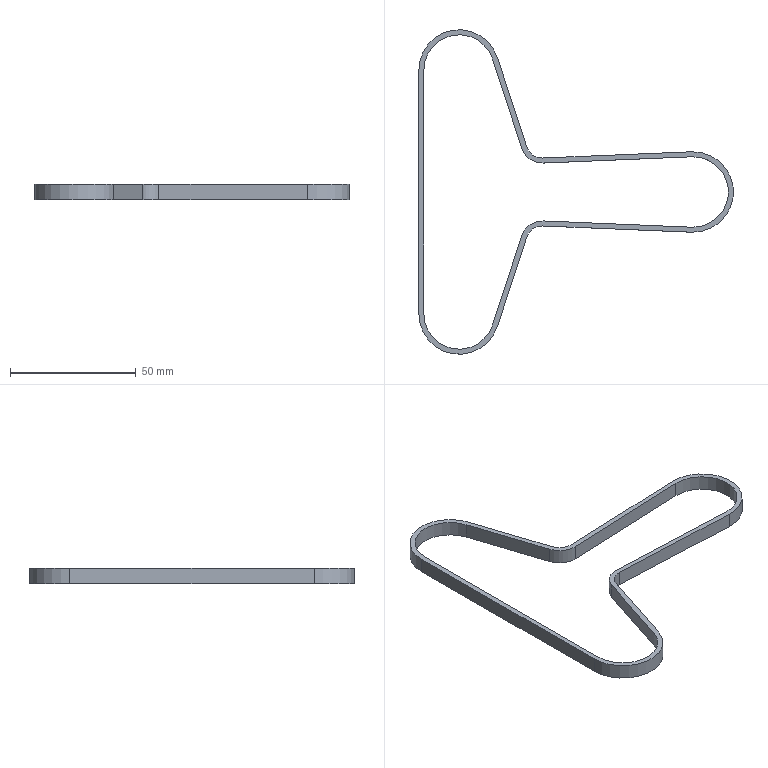Part | STEP file | HTUN453S3M-60 | 1 solid | 22 faces | box 125 x 129 x 6 mm | volume 5310 mm3 | plane 12 | cylinder 10 | commonest cylinder face diameters 28 x3 32 x3 13 x2 17 x2
STEP:
#1=CARTESIAN_POINT('',(92.329,-15.986,6.));
#2=VERTEX_POINT('',#1);
#3=CARTESIAN_POINT('',(92.329,15.986,6.));
#4=VERTEX_POINT('',#3);
#5=CARTESIAN_POINT('',(93.,0.,6.));
#6=DIRECTION('',(0.,0.,1.));
#7=DIRECTION('',(1.,0.,0.));
#8=AXIS2_PLACEMENT_3D('',#5,#6,#7);
#9=CIRCLE('',#8,16.);
#10=EDGE_CURVE('',#2,#4,#9,.T.);
#11=ORIENTED_EDGE('',*,*,#10,.T.);
#12=CARTESIAN_POINT('',(33.273,13.506,6.));
#13=VERTEX_POINT('',#12);
#14=CARTESIAN_POINT('',(92.329,15.986,6.));
#15=DIRECTION('',(-0.9991,-0.04196,0.));
#16=VECTOR('',#15,1000.);
#17=LINE('',#14,#16);
#18=EDGE_CURVE('',#4,#13,#17,.T.);
#19=ORIENTED_EDGE('',*,*,#18,.T.);
#20=CARTESIAN_POINT('',(26.822,17.978,6.));
#21=VERTEX_POINT('',#20);
#22=CARTESIAN_POINT('',(33.,20.,6.));
#23=DIRECTION('',(0.,0.,-1.));
#24=DIRECTION('',(1.,0.,0.));
#25=AXIS2_PLACEMENT_3D('',#22,#23,#24);
#26=CIRCLE('',#25,6.5);
#27=EDGE_CURVE('',#13,#21,#26,.T.);
#28=ORIENTED_EDGE('',*,*,#27,.T.);
#29=CARTESIAN_POINT('',(15.207,53.476,6.));
#30=VERTEX_POINT('',#29);
#31=CARTESIAN_POINT('',(15.207,53.476,6.));
#32=DIRECTION('',(-0.311,0.9504,0.));
#33=VECTOR('',#32,1000.);
#34=LINE('',#31,#33);
#35=EDGE_CURVE('',#21,#30,#34,.T.);
#36=ORIENTED_EDGE('',*,*,#35,.T.);
#37=CARTESIAN_POINT('',(-16.,48.5,6.));
#38=VERTEX_POINT('',#37);
#39=CARTESIAN_POINT('',(0.,48.5,6.));
#40=DIRECTION('',(0.,0.,1.));
#41=DIRECTION('',(1.,0.,0.));
#42=AXIS2_PLACEMENT_3D('',#39,#40,#41);
#43=CIRCLE('',#42,16.);
#44=EDGE_CURVE('',#30,#38,#43,.T.);
#45=ORIENTED_EDGE('',*,*,#44,.T.);
#46=CARTESIAN_POINT('',(-16.,-48.5,6.));
#47=VERTEX_POINT('',#46);
#48=CARTESIAN_POINT('',(-16.,48.5,6.));
#49=DIRECTION('',(0.,-1.,0.));
#50=VECTOR('',#49,1000.);
#51=LINE('',#48,#50);
#52=EDGE_CURVE('',#38,#47,#51,.T.);
#53=ORIENTED_EDGE('',*,*,#52,.T.);
#54=CARTESIAN_POINT('',(15.207,-53.476,6.));
#55=VERTEX_POINT('',#54);
#56=CARTESIAN_POINT('',(0.,-48.5,6.));
#57=DIRECTION('',(0.,0.,1.));
#58=DIRECTION('',(-1.,0.,0.));
#59=AXIS2_PLACEMENT_3D('',#56,#57,#58);
#60=CIRCLE('',#59,16.);
#61=EDGE_CURVE('',#47,#55,#60,.T.);
#62=ORIENTED_EDGE('',*,*,#61,.T.);
#63=CARTESIAN_POINT('',(26.822,-17.978,6.));
#64=VERTEX_POINT('',#63);
#65=CARTESIAN_POINT('',(15.207,-53.476,6.));
#66=DIRECTION('',(0.311,0.9504,0.));
#67=VECTOR('',#66,1000.);
#68=LINE('',#65,#67);
#69=EDGE_CURVE('',#55,#64,#68,.T.);
#70=ORIENTED_EDGE('',*,*,#69,.T.);
#71=CARTESIAN_POINT('',(33.273,-13.506,6.));
#72=VERTEX_POINT('',#71);
#73=CARTESIAN_POINT('',(33.,-20.,6.));
#74=DIRECTION('',(0.,0.,-1.));
#75=DIRECTION('',(-1.,0.,0.));
#76=AXIS2_PLACEMENT_3D('',#73,#74,#75);
#77=CIRCLE('',#76,6.5);
#78=EDGE_CURVE('',#64,#72,#77,.T.);
#79=ORIENTED_EDGE('',*,*,#78,.T.);
#80=CARTESIAN_POINT('',(92.329,-15.986,6.));
#81=DIRECTION('',(0.9991,-0.04196,0.));
#82=VECTOR('',#81,1000.);
#83=LINE('',#80,#82);
#84=EDGE_CURVE('',#72,#2,#83,.T.);
#85=ORIENTED_EDGE('',*,*,#84,.T.);
#86=EDGE_LOOP('',(#11,#19,#28,#36,#45,#53,#62,#70,#79,#85));
#87=FACE_OUTER_BOUND('',#86,.T.);
#88=CARTESIAN_POINT('',(92.413,13.988,6.));
#89=VERTEX_POINT('',#88);
#90=CARTESIAN_POINT('',(33.357,11.507,6.));
#91=VERTEX_POINT('',#90);
#92=CARTESIAN_POINT('',(92.413,13.988,6.));
#93=DIRECTION('',(-0.9991,-0.04196,0.));
#94=VECTOR('',#93,1000.);
#95=LINE('',#92,#94);
#96=EDGE_CURVE('',#89,#91,#95,.T.);
#97=ORIENTED_EDGE('',*,*,#96,.F.);
#98=CARTESIAN_POINT('',(92.413,-13.988,6.));
#99=VERTEX_POINT('',#98);
#100=CARTESIAN_POINT('',(93.,0.,6.));
#101=DIRECTION('',(0.,0.,1.));
#102=DIRECTION('',(1.,0.,0.));
#103=AXIS2_PLACEMENT_3D('',#100,#101,#102);
#104=CIRCLE('',#103,14.);
#105=EDGE_CURVE('',#99,#89,#104,.T.);
#106=ORIENTED_EDGE('',*,*,#105,.F.);
#107=CARTESIAN_POINT('',(33.357,-11.507,6.));
#108=VERTEX_POINT('',#107);
#109=CARTESIAN_POINT('',(92.413,-13.988,6.));
#110=DIRECTION('',(0.9991,-0.04196,0.));
#111=VECTOR('',#110,1000.);
#112=LINE('',#109,#111);
#113=EDGE_CURVE('',#108,#99,#112,.T.);
#114=ORIENTED_EDGE('',*,*,#113,.F.);
#115=CARTESIAN_POINT('',(24.922,-17.356,6.));
#116=VERTEX_POINT('',#115);
#117=CARTESIAN_POINT('',(33.,-20.,6.));
#118=DIRECTION('',(0.,0.,-1.));
#119=DIRECTION('',(-1.,0.,0.));
#120=AXIS2_PLACEMENT_3D('',#117,#118,#119);
#121=CIRCLE('',#120,8.5);
#122=EDGE_CURVE('',#116,#108,#121,.T.);
#123=ORIENTED_EDGE('',*,*,#122,.F.);
#124=CARTESIAN_POINT('',(13.306,-52.854,6.));
#125=VERTEX_POINT('',#124);
#126=CARTESIAN_POINT('',(13.306,-52.854,6.));
#127=DIRECTION('',(0.311,0.9504,0.));
#128=VECTOR('',#127,1000.);
#129=LINE('',#126,#128);
#130=EDGE_CURVE('',#125,#116,#129,.T.);
#131=ORIENTED_EDGE('',*,*,#130,.F.);
#132=CARTESIAN_POINT('',(-14.,-48.5,6.));
#133=VERTEX_POINT('',#132);
#134=CARTESIAN_POINT('',(0.,-48.5,6.));
#135=DIRECTION('',(0.,0.,1.));
#136=DIRECTION('',(-1.,0.,0.));
#137=AXIS2_PLACEMENT_3D('',#134,#135,#136);
#138=CIRCLE('',#137,14.);
#139=EDGE_CURVE('',#133,#125,#138,.T.);
#140=ORIENTED_EDGE('',*,*,#139,.F.);
#141=CARTESIAN_POINT('',(-14.,48.5,6.));
#142=VERTEX_POINT('',#141);
#143=CARTESIAN_POINT('',(-14.,48.5,6.));
#144=DIRECTION('',(0.,-1.,0.));
#145=VECTOR('',#144,1000.);
#146=LINE('',#143,#145);
#147=EDGE_CURVE('',#142,#133,#146,.T.);
#148=ORIENTED_EDGE('',*,*,#147,.F.);
#149=CARTESIAN_POINT('',(13.306,52.854,6.));
#150=VERTEX_POINT('',#149);
#151=CARTESIAN_POINT('',(0.,48.5,6.));
#152=DIRECTION('',(0.,0.,1.));
#153=DIRECTION('',(1.,0.,0.));
#154=AXIS2_PLACEMENT_3D('',#151,#152,#153);
#155=CIRCLE('',#154,14.);
#156=EDGE_CURVE('',#150,#142,#155,.T.);
#157=ORIENTED_EDGE('',*,*,#156,.F.);
#158=CARTESIAN_POINT('',(24.922,17.356,6.));
#159=VERTEX_POINT('',#158);
#160=CARTESIAN_POINT('',(13.306,52.854,6.));
#161=DIRECTION('',(-0.311,0.9504,0.));
#162=VECTOR('',#161,1000.);
#163=LINE('',#160,#162);
#164=EDGE_CURVE('',#159,#150,#163,.T.);
#165=ORIENTED_EDGE('',*,*,#164,.F.);
#166=CARTESIAN_POINT('',(33.,20.,6.));
#167=DIRECTION('',(0.,0.,-1.));
#168=DIRECTION('',(1.,0.,0.));
#169=AXIS2_PLACEMENT_3D('',#166,#167,#168);
#170=CIRCLE('',#169,8.5);
#171=EDGE_CURVE('',#91,#159,#170,.T.);
#172=ORIENTED_EDGE('',*,*,#171,.F.);
#173=EDGE_LOOP('',(#97,#106,#114,#123,#131,#140,#148,#157,#165,#172));
#174=FACE_BOUND('',#173,.T.);
#175=CARTESIAN_POINT('',(93.,0.,6.));
#176=DIRECTION('',(0.,0.,1.));
#177=DIRECTION('',(1.,0.,0.));
#178=AXIS2_PLACEMENT_3D('',#175,#176,#177);
#179=PLANE('',#178);
#180=ADVANCED_FACE('',(#87,#174),#179,.T.);
#181=CARTESIAN_POINT('',(92.329,-15.986,0.));
#182=VERTEX_POINT('',#181);
#183=CARTESIAN_POINT('',(92.329,15.986,0.));
#184=VERTEX_POINT('',#183);
#185=CARTESIAN_POINT('',(93.,0.,0.));
#186=DIRECTION('',(0.,0.,1.));
#187=DIRECTION('',(1.,0.,0.));
#188=AXIS2_PLACEMENT_3D('',#185,#186,#187);
#189=CIRCLE('',#188,16.);
#190=EDGE_CURVE('',#182,#184,#189,.T.);
#191=ORIENTED_EDGE('',*,*,#190,.F.);
#192=CARTESIAN_POINT('',(33.273,-13.506,0.));
#193=VERTEX_POINT('',#192);
#194=CARTESIAN_POINT('',(92.329,-15.986,0.));
#195=DIRECTION('',(0.9991,-0.04196,0.));
#196=VECTOR('',#195,1000.);
#197=LINE('',#194,#196);
#198=EDGE_CURVE('',#193,#182,#197,.T.);
#199=ORIENTED_EDGE('',*,*,#198,.F.);
#200=CARTESIAN_POINT('',(26.822,-17.978,0.));
#201=VERTEX_POINT('',#200);
#202=CARTESIAN_POINT('',(33.,-20.,0.));
#203=DIRECTION('',(0.,0.,-1.));
#204=DIRECTION('',(-1.,0.,0.));
#205=AXIS2_PLACEMENT_3D('',#202,#203,#204);
#206=CIRCLE('',#205,6.5);
#207=EDGE_CURVE('',#201,#193,#206,.T.);
#208=ORIENTED_EDGE('',*,*,#207,.F.);
#209=CARTESIAN_POINT('',(15.207,-53.476,0.));
#210=VERTEX_POINT('',#209);
#211=CARTESIAN_POINT('',(15.207,-53.476,0.));
#212=DIRECTION('',(0.311,0.9504,0.));
#213=VECTOR('',#212,1000.);
#214=LINE('',#211,#213);
#215=EDGE_CURVE('',#210,#201,#214,.T.);
#216=ORIENTED_EDGE('',*,*,#215,.F.);
#217=CARTESIAN_POINT('',(-16.,-48.5,0.));
#218=VERTEX_POINT('',#217);
#219=CARTESIAN_POINT('',(0.,-48.5,0.));
#220=DIRECTION('',(0.,0.,1.));
#221=DIRECTION('',(-1.,0.,0.));
#222=AXIS2_PLACEMENT_3D('',#219,#220,#221);
#223=CIRCLE('',#222,16.);
#224=EDGE_CURVE('',#218,#210,#223,.T.);
#225=ORIENTED_EDGE('',*,*,#224,.F.);
#226=CARTESIAN_POINT('',(-16.,48.5,0.));
#227=VERTEX_POINT('',#226);
#228=CARTESIAN_POINT('',(-16.,48.5,0.));
#229=DIRECTION('',(0.,-1.,0.));
#230=VECTOR('',#229,1000.);
#231=LINE('',#228,#230);
#232=EDGE_CURVE('',#227,#218,#231,.T.);
#233=ORIENTED_EDGE('',*,*,#232,.F.);
#234=CARTESIAN_POINT('',(15.207,53.476,0.));
#235=VERTEX_POINT('',#234);
#236=CARTESIAN_POINT('',(0.,48.5,0.));
#237=DIRECTION('',(0.,0.,1.));
#238=DIRECTION('',(1.,0.,0.));
#239=AXIS2_PLACEMENT_3D('',#236,#237,#238);
#240=CIRCLE('',#239,16.);
#241=EDGE_CURVE('',#235,#227,#240,.T.);
#242=ORIENTED_EDGE('',*,*,#241,.F.);
#243=CARTESIAN_POINT('',(26.822,17.978,0.));
#244=VERTEX_POINT('',#243);
#245=CARTESIAN_POINT('',(15.207,53.476,0.));
#246=DIRECTION('',(-0.311,0.9504,0.));
#247=VECTOR('',#246,1000.);
#248=LINE('',#245,#247);
#249=EDGE_CURVE('',#244,#235,#248,.T.);
#250=ORIENTED_EDGE('',*,*,#249,.F.);
#251=CARTESIAN_POINT('',(33.273,13.506,0.));
#252=VERTEX_POINT('',#251);
#253=CARTESIAN_POINT('',(33.,20.,0.));
#254=DIRECTION('',(0.,0.,-1.));
#255=DIRECTION('',(1.,0.,0.));
#256=AXIS2_PLACEMENT_3D('',#253,#254,#255);
#257=CIRCLE('',#256,6.5);
#258=EDGE_CURVE('',#252,#244,#257,.T.);
#259=ORIENTED_EDGE('',*,*,#258,.F.);
#260=CARTESIAN_POINT('',(92.329,15.986,0.));
#261=DIRECTION('',(-0.9991,-0.04196,0.));
#262=VECTOR('',#261,1000.);
#263=LINE('',#260,#262);
#264=EDGE_CURVE('',#184,#252,#263,.T.);
#265=ORIENTED_EDGE('',*,*,#264,.F.);
#266=EDGE_LOOP('',(#191,#199,#208,#216,#225,#233,#242,#250,#259,#265));
#267=FACE_OUTER_BOUND('',#266,.T.);
#268=CARTESIAN_POINT('',(92.413,-13.988,0.));
#269=VERTEX_POINT('',#268);
#270=CARTESIAN_POINT('',(92.413,13.988,0.));
#271=VERTEX_POINT('',#270);
#272=CARTESIAN_POINT('',(93.,0.,0.));
#273=DIRECTION('',(0.,0.,1.));
#274=DIRECTION('',(1.,0.,0.));
#275=AXIS2_PLACEMENT_3D('',#272,#273,#274);
#276=CIRCLE('',#275,14.);
#277=EDGE_CURVE('',#269,#271,#276,.T.);
#278=ORIENTED_EDGE('',*,*,#277,.T.);
#279=CARTESIAN_POINT('',(33.357,11.507,0.));
#280=VERTEX_POINT('',#279);
#281=CARTESIAN_POINT('',(92.413,13.988,0.));
#282=DIRECTION('',(-0.9991,-0.04196,0.));
#283=VECTOR('',#282,1000.);
#284=LINE('',#281,#283);
#285=EDGE_CURVE('',#271,#280,#284,.T.);
#286=ORIENTED_EDGE('',*,*,#285,.T.);
#287=CARTESIAN_POINT('',(24.922,17.356,0.));
#288=VERTEX_POINT('',#287);
#289=CARTESIAN_POINT('',(33.,20.,0.));
#290=DIRECTION('',(0.,0.,-1.));
#291=DIRECTION('',(1.,0.,0.));
#292=AXIS2_PLACEMENT_3D('',#289,#290,#291);
#293=CIRCLE('',#292,8.5);
#294=EDGE_CURVE('',#280,#288,#293,.T.);
#295=ORIENTED_EDGE('',*,*,#294,.T.);
#296=CARTESIAN_POINT('',(13.306,52.854,0.));
#297=VERTEX_POINT('',#296);
#298=CARTESIAN_POINT('',(13.306,52.854,0.));
#299=DIRECTION('',(-0.311,0.9504,0.));
#300=VECTOR('',#299,1000.);
#301=LINE('',#298,#300);
#302=EDGE_CURVE('',#288,#297,#301,.T.);
#303=ORIENTED_EDGE('',*,*,#302,.T.);
#304=CARTESIAN_POINT('',(-14.,48.5,0.));
#305=VERTEX_POINT('',#304);
#306=CARTESIAN_POINT('',(0.,48.5,0.));
#307=DIRECTION('',(0.,0.,1.));
#308=DIRECTION('',(1.,0.,0.));
#309=AXIS2_PLACEMENT_3D('',#306,#307,#308);
#310=CIRCLE('',#309,14.);
#311=EDGE_CURVE('',#297,#305,#310,.T.);
#312=ORIENTED_EDGE('',*,*,#311,.T.);
#313=CARTESIAN_POINT('',(-14.,-48.5,0.));
#314=VERTEX_POINT('',#313);
#315=CARTESIAN_POINT('',(-14.,48.5,0.));
#316=DIRECTION('',(0.,-1.,0.));
#317=VECTOR('',#316,1000.);
#318=LINE('',#315,#317);
#319=EDGE_CURVE('',#305,#314,#318,.T.);
#320=ORIENTED_EDGE('',*,*,#319,.T.);
#321=CARTESIAN_POINT('',(13.306,-52.854,0.));
#322=VERTEX_POINT('',#321);
#323=CARTESIAN_POINT('',(0.,-48.5,0.));
#324=DIRECTION('',(0.,0.,1.));
#325=DIRECTION('',(-1.,0.,0.));
#326=AXIS2_PLACEMENT_3D('',#323,#324,#325);
#327=CIRCLE('',#326,14.);
#328=EDGE_CURVE('',#314,#322,#327,.T.);
#329=ORIENTED_EDGE('',*,*,#328,.T.);
#330=CARTESIAN_POINT('',(24.922,-17.356,0.));
#331=VERTEX_POINT('',#330);
#332=CARTESIAN_POINT('',(13.306,-52.854,0.));
#333=DIRECTION('',(0.311,0.9504,0.));
#334=VECTOR('',#333,1000.);
#335=LINE('',#332,#334);
#336=EDGE_CURVE('',#322,#331,#335,.T.);
#337=ORIENTED_EDGE('',*,*,#336,.T.);
#338=CARTESIAN_POINT('',(33.357,-11.507,0.));
#339=VERTEX_POINT('',#338);
#340=CARTESIAN_POINT('',(33.,-20.,0.));
#341=DIRECTION('',(0.,0.,-1.));
#342=DIRECTION('',(-1.,0.,0.));
#343=AXIS2_PLACEMENT_3D('',#340,#341,#342);
#344=CIRCLE('',#343,8.5);
#345=EDGE_CURVE('',#331,#339,#344,.T.);
#346=ORIENTED_EDGE('',*,*,#345,.T.);
#347=CARTESIAN_POINT('',(92.413,-13.988,0.));
#348=DIRECTION('',(0.9991,-0.04196,0.));
#349=VECTOR('',#348,1000.);
#350=LINE('',#347,#349);
#351=EDGE_CURVE('',#339,#269,#350,.T.);
#352=ORIENTED_EDGE('',*,*,#351,.T.);
#353=EDGE_LOOP('',(#278,#286,#295,#303,#312,#320,#329,#337,#346,#352));
#354=FACE_BOUND('',#353,.T.);
#355=CARTESIAN_POINT('',(93.,0.,0.));
#356=DIRECTION('',(0.,0.,1.));
#357=DIRECTION('',(1.,0.,0.));
#358=AXIS2_PLACEMENT_3D('',#355,#356,#357);
#359=PLANE('',#358);
#360=ADVANCED_FACE('',(#267,#354),#359,.F.);
#361=ORIENTED_EDGE('',*,*,#190,.T.);
#362=CARTESIAN_POINT('',(92.329,15.986,6.));
#363=DIRECTION('',(0.,0.,-1.));
#364=VECTOR('',#363,1000.);
#365=LINE('',#362,#364);
#366=EDGE_CURVE('',#4,#184,#365,.T.);
#367=ORIENTED_EDGE('',*,*,#366,.F.);
#368=ORIENTED_EDGE('',*,*,#10,.F.);
#369=CARTESIAN_POINT('',(92.329,-15.986,6.));
#370=DIRECTION('',(0.,0.,-1.));
#371=VECTOR('',#370,1000.);
#372=LINE('',#369,#371);
#373=EDGE_CURVE('',#2,#182,#372,.T.);
#374=ORIENTED_EDGE('',*,*,#373,.T.);
#375=EDGE_LOOP('',(#361,#367,#368,#374));
#376=FACE_OUTER_BOUND('',#375,.T.);
#377=CARTESIAN_POINT('',(93.,0.,6.));
#378=DIRECTION('',(0.,0.,-1.));
#379=DIRECTION('',(-1.,0.,0.));
#380=AXIS2_PLACEMENT_3D('',#377,#378,#379);
#381=CYLINDRICAL_SURFACE('',#380,16.);
#382=ADVANCED_FACE('',(#376),#381,.T.);
#383=ORIENTED_EDGE('',*,*,#264,.T.);
#384=CARTESIAN_POINT('',(33.273,13.506,6.));
#385=DIRECTION('',(0.,0.,-1.));
#386=VECTOR('',#385,1000.);
#387=LINE('',#384,#386);
#388=EDGE_CURVE('',#13,#252,#387,.T.);
#389=ORIENTED_EDGE('',*,*,#388,.F.);
#390=ORIENTED_EDGE('',*,*,#18,.F.);
#391=ORIENTED_EDGE('',*,*,#366,.T.);
#392=EDGE_LOOP('',(#383,#389,#390,#391));
#393=FACE_OUTER_BOUND('',#392,.T.);
#394=CARTESIAN_POINT('',(92.329,15.986,6.));
#395=DIRECTION('',(0.04196,-0.9991,0.));
#396=DIRECTION('',(0.9991,0.04196,0.));
#397=AXIS2_PLACEMENT_3D('',#394,#395,#396);
#398=PLANE('',#397);
#399=ADVANCED_FACE('',(#393),#398,.F.);
#400=ORIENTED_EDGE('',*,*,#258,.T.);
#401=CARTESIAN_POINT('',(26.822,17.978,6.));
#402=DIRECTION('',(0.,0.,-1.));
#403=VECTOR('',#402,1000.);
#404=LINE('',#401,#403);
#405=EDGE_CURVE('',#21,#244,#404,.T.);
#406=ORIENTED_EDGE('',*,*,#405,.F.);
#407=ORIENTED_EDGE('',*,*,#27,.F.);
#408=ORIENTED_EDGE('',*,*,#388,.T.);
#409=EDGE_LOOP('',(#400,#406,#407,#408));
#410=FACE_OUTER_BOUND('',#409,.T.);
#411=CARTESIAN_POINT('',(33.,20.,6.));
#412=DIRECTION('',(0.,0.,-1.));
#413=DIRECTION('',(-1.,0.,0.));
#414=AXIS2_PLACEMENT_3D('',#411,#412,#413);
#415=CYLINDRICAL_SURFACE('',#414,6.5);
#416=ADVANCED_FACE('',(#410),#415,.F.);
#417=ORIENTED_EDGE('',*,*,#249,.T.);
#418=CARTESIAN_POINT('',(15.207,53.476,6.));
#419=DIRECTION('',(0.,0.,-1.));
#420=VECTOR('',#419,1000.);
#421=LINE('',#418,#420);
#422=EDGE_CURVE('',#30,#235,#421,.T.);
#423=ORIENTED_EDGE('',*,*,#422,.F.);
#424=ORIENTED_EDGE('',*,*,#35,.F.);
#425=ORIENTED_EDGE('',*,*,#405,.T.);
#426=EDGE_LOOP('',(#417,#423,#424,#425));
#427=FACE_OUTER_BOUND('',#426,.T.);
#428=CARTESIAN_POINT('',(15.207,53.476,6.));
#429=DIRECTION('',(-0.9504,-0.311,0.));
#430=DIRECTION('',(0.311,-0.9504,0.));
#431=AXIS2_PLACEMENT_3D('',#428,#429,#430);
#432=PLANE('',#431);
#433=ADVANCED_FACE('',(#427),#432,.F.);
#434=ORIENTED_EDGE('',*,*,#241,.T.);
#435=CARTESIAN_POINT('',(-16.,48.5,6.));
#436=DIRECTION('',(0.,0.,-1.));
#437=VECTOR('',#436,1000.);
#438=LINE('',#435,#437);
#439=EDGE_CURVE('',#38,#227,#438,.T.);
#440=ORIENTED_EDGE('',*,*,#439,.F.);
#441=ORIENTED_EDGE('',*,*,#44,.F.);
#442=ORIENTED_EDGE('',*,*,#422,.T.);
#443=EDGE_LOOP('',(#434,#440,#441,#442));
#444=FACE_OUTER_BOUND('',#443,.T.);
#445=CARTESIAN_POINT('',(0.,48.5,6.));
#446=DIRECTION('',(0.,0.,-1.));
#447=DIRECTION('',(-1.,0.,0.));
#448=AXIS2_PLACEMENT_3D('',#445,#446,#447);
#449=CYLINDRICAL_SURFACE('',#448,16.);
#450=ADVANCED_FACE('',(#444),#449,.T.);
#451=ORIENTED_EDGE('',*,*,#232,.T.);
#452=CARTESIAN_POINT('',(-16.,-48.5,6.));
#453=DIRECTION('',(0.,0.,-1.));
#454=VECTOR('',#453,1000.);
#455=LINE('',#452,#454);
#456=EDGE_CURVE('',#47,#218,#455,.T.);
#457=ORIENTED_EDGE('',*,*,#456,.F.);
#458=ORIENTED_EDGE('',*,*,#52,.F.);
#459=ORIENTED_EDGE('',*,*,#439,.T.);
#460=EDGE_LOOP('',(#451,#457,#458,#459));
#461=FACE_OUTER_BOUND('',#460,.T.);
#462=CARTESIAN_POINT('',(-16.,48.5,6.));
#463=DIRECTION('',(1.,0.,0.));
#464=DIRECTION('',(0.,1.,0.));
#465=AXIS2_PLACEMENT_3D('',#462,#463,#464);
#466=PLANE('',#465);
#467=ADVANCED_FACE('',(#461),#466,.F.);
#468=ORIENTED_EDGE('',*,*,#224,.T.);
#469=CARTESIAN_POINT('',(15.207,-53.476,6.));
#470=DIRECTION('',(0.,0.,-1.));
#471=VECTOR('',#470,1000.);
#472=LINE('',#469,#471);
#473=EDGE_CURVE('',#55,#210,#472,.T.);
#474=ORIENTED_EDGE('',*,*,#473,.F.);
#475=ORIENTED_EDGE('',*,*,#61,.F.);
#476=ORIENTED_EDGE('',*,*,#456,.T.);
#477=EDGE_LOOP('',(#468,#474,#475,#476));
#478=FACE_OUTER_BOUND('',#477,.T.);
#479=CARTESIAN_POINT('',(0.,-48.5,6.));
#480=DIRECTION('',(0.,0.,-1.));
#481=DIRECTION('',(-1.,0.,0.));
#482=AXIS2_PLACEMENT_3D('',#479,#480,#481);
#483=CYLINDRICAL_SURFACE('',#482,16.);
#484=ADVANCED_FACE('',(#478),#483,.T.);
#485=ORIENTED_EDGE('',*,*,#215,.T.);
#486=CARTESIAN_POINT('',(26.822,-17.978,6.));
#487=DIRECTION('',(0.,0.,-1.));
#488=VECTOR('',#487,1000.);
#489=LINE('',#486,#488);
#490=EDGE_CURVE('',#64,#201,#489,.T.);
#491=ORIENTED_EDGE('',*,*,#490,.F.);
#492=ORIENTED_EDGE('',*,*,#69,.F.);
#493=ORIENTED_EDGE('',*,*,#473,.T.);
#494=EDGE_LOOP('',(#485,#491,#492,#493));
#495=FACE_OUTER_BOUND('',#494,.T.);
#496=CARTESIAN_POINT('',(15.207,-53.476,6.));
#497=DIRECTION('',(-0.9504,0.311,0.));
#498=DIRECTION('',(-0.311,-0.9504,0.));
#499=AXIS2_PLACEMENT_3D('',#496,#497,#498);
#500=PLANE('',#499);
#501=ADVANCED_FACE('',(#495),#500,.F.);
#502=ORIENTED_EDGE('',*,*,#207,.T.);
#503=CARTESIAN_POINT('',(33.273,-13.506,6.));
#504=DIRECTION('',(0.,0.,-1.));
#505=VECTOR('',#504,1000.);
#506=LINE('',#503,#505);
#507=EDGE_CURVE('',#72,#193,#506,.T.);
#508=ORIENTED_EDGE('',*,*,#507,.F.);
#509=ORIENTED_EDGE('',*,*,#78,.F.);
#510=ORIENTED_EDGE('',*,*,#490,.T.);
#511=EDGE_LOOP('',(#502,#508,#509,#510));
#512=FACE_OUTER_BOUND('',#511,.T.);
#513=CARTESIAN_POINT('',(33.,-20.,6.));
#514=DIRECTION('',(0.,0.,-1.));
#515=DIRECTION('',(-1.,0.,0.));
#516=AXIS2_PLACEMENT_3D('',#513,#514,#515);
#517=CYLINDRICAL_SURFACE('',#516,6.5);
#518=ADVANCED_FACE('',(#512),#517,.F.);
#519=ORIENTED_EDGE('',*,*,#198,.T.);
#520=ORIENTED_EDGE('',*,*,#373,.F.);
#521=ORIENTED_EDGE('',*,*,#84,.F.);
#522=ORIENTED_EDGE('',*,*,#507,.T.);
#523=EDGE_LOOP('',(#519,#520,#521,#522));
#524=FACE_OUTER_BOUND('',#523,.T.);
#525=CARTESIAN_POINT('',(92.329,-15.986,6.));
#526=DIRECTION('',(0.04196,0.9991,0.));
#527=DIRECTION('',(-0.9991,0.04196,0.));
#528=AXIS2_PLACEMENT_3D('',#525,#526,#527);
#529=PLANE('',#528);
#530=ADVANCED_FACE('',(#524),#529,.F.);
#531=ORIENTED_EDGE('',*,*,#277,.F.);
#532=CARTESIAN_POINT('',(92.413,-13.988,6.));
#533=DIRECTION('',(0.,0.,-1.));
#534=VECTOR('',#533,1000.);
#535=LINE('',#532,#534);
#536=EDGE_CURVE('',#99,#269,#535,.T.);
#537=ORIENTED_EDGE('',*,*,#536,.F.);
#538=ORIENTED_EDGE('',*,*,#105,.T.);
#539=CARTESIAN_POINT('',(92.413,13.988,6.));
#540=DIRECTION('',(0.,0.,-1.));
#541=VECTOR('',#540,1000.);
#542=LINE('',#539,#541);
#543=EDGE_CURVE('',#89,#271,#542,.T.);
#544=ORIENTED_EDGE('',*,*,#543,.T.);
#545=EDGE_LOOP('',(#531,#537,#538,#544));
#546=FACE_OUTER_BOUND('',#545,.T.);
#547=CARTESIAN_POINT('',(93.,0.,6.));
#548=DIRECTION('',(0.,0.,-1.));
#549=DIRECTION('',(-1.,0.,0.));
#550=AXIS2_PLACEMENT_3D('',#547,#548,#549);
#551=CYLINDRICAL_SURFACE('',#550,14.);
#552=ADVANCED_FACE('',(#546),#551,.F.);
#553=ORIENTED_EDGE('',*,*,#285,.F.);
#554=ORIENTED_EDGE('',*,*,#543,.F.);
#555=ORIENTED_EDGE('',*,*,#96,.T.);
#556=CARTESIAN_POINT('',(33.357,11.507,6.));
#557=DIRECTION('',(0.,0.,-1.));
#558=VECTOR('',#557,1000.);
#559=LINE('',#556,#558);
#560=EDGE_CURVE('',#91,#280,#559,.T.);
#561=ORIENTED_EDGE('',*,*,#560,.T.);
#562=EDGE_LOOP('',(#553,#554,#555,#561));
#563=FACE_OUTER_BOUND('',#562,.T.);
#564=CARTESIAN_POINT('',(92.413,13.988,6.));
#565=DIRECTION('',(0.04196,-0.9991,0.));
#566=DIRECTION('',(0.9991,0.04196,0.));
#567=AXIS2_PLACEMENT_3D('',#564,#565,#566);
#568=PLANE('',#567);
#569=ADVANCED_FACE('',(#563),#568,.T.);
#570=ORIENTED_EDGE('',*,*,#294,.F.);
#571=ORIENTED_EDGE('',*,*,#560,.F.);
#572=ORIENTED_EDGE('',*,*,#171,.T.);
#573=CARTESIAN_POINT('',(24.922,17.356,6.));
#574=DIRECTION('',(0.,0.,-1.));
#575=VECTOR('',#574,1000.);
#576=LINE('',#573,#575);
#577=EDGE_CURVE('',#159,#288,#576,.T.);
#578=ORIENTED_EDGE('',*,*,#577,.T.);
#579=EDGE_LOOP('',(#570,#571,#572,#578));
#580=FACE_OUTER_BOUND('',#579,.T.);
#581=CARTESIAN_POINT('',(33.,20.,6.));
#582=DIRECTION('',(0.,0.,-1.));
#583=DIRECTION('',(-1.,0.,0.));
#584=AXIS2_PLACEMENT_3D('',#581,#582,#583);
#585=CYLINDRICAL_SURFACE('',#584,8.5);
#586=ADVANCED_FACE('',(#580),#585,.T.);
#587=ORIENTED_EDGE('',*,*,#302,.F.);
#588=ORIENTED_EDGE('',*,*,#577,.F.);
#589=ORIENTED_EDGE('',*,*,#164,.T.);
#590=CARTESIAN_POINT('',(13.306,52.854,6.));
#591=DIRECTION('',(0.,0.,-1.));
#592=VECTOR('',#591,1000.);
#593=LINE('',#590,#592);
#594=EDGE_CURVE('',#150,#297,#593,.T.);
#595=ORIENTED_EDGE('',*,*,#594,.T.);
#596=EDGE_LOOP('',(#587,#588,#589,#595));
#597=FACE_OUTER_BOUND('',#596,.T.);
#598=CARTESIAN_POINT('',(13.306,52.854,6.));
#599=DIRECTION('',(-0.9504,-0.311,0.));
#600=DIRECTION('',(0.311,-0.9504,0.));
#601=AXIS2_PLACEMENT_3D('',#598,#599,#600);
#602=PLANE('',#601);
#603=ADVANCED_FACE('',(#597),#602,.T.);
#604=ORIENTED_EDGE('',*,*,#311,.F.);
#605=ORIENTED_EDGE('',*,*,#594,.F.);
#606=ORIENTED_EDGE('',*,*,#156,.T.);
#607=CARTESIAN_POINT('',(-14.,48.5,6.));
#608=DIRECTION('',(0.,0.,-1.));
#609=VECTOR('',#608,1000.);
#610=LINE('',#607,#609);
#611=EDGE_CURVE('',#142,#305,#610,.T.);
#612=ORIENTED_EDGE('',*,*,#611,.T.);
#613=EDGE_LOOP('',(#604,#605,#606,#612));
#614=FACE_OUTER_BOUND('',#613,.T.);
#615=CARTESIAN_POINT('',(0.,48.5,6.));
#616=DIRECTION('',(0.,0.,-1.));
#617=DIRECTION('',(-1.,0.,0.));
#618=AXIS2_PLACEMENT_3D('',#615,#616,#617);
#619=CYLINDRICAL_SURFACE('',#618,14.);
#620=ADVANCED_FACE('',(#614),#619,.F.);
#621=ORIENTED_EDGE('',*,*,#319,.F.);
#622=ORIENTED_EDGE('',*,*,#611,.F.);
#623=ORIENTED_EDGE('',*,*,#147,.T.);
#624=CARTESIAN_POINT('',(-14.,-48.5,6.));
#625=DIRECTION('',(0.,0.,-1.));
#626=VECTOR('',#625,1000.);
#627=LINE('',#624,#626);
#628=EDGE_CURVE('',#133,#314,#627,.T.);
#629=ORIENTED_EDGE('',*,*,#628,.T.);
#630=EDGE_LOOP('',(#621,#622,#623,#629));
#631=FACE_OUTER_BOUND('',#630,.T.);
#632=CARTESIAN_POINT('',(-14.,48.5,6.));
#633=DIRECTION('',(1.,0.,0.));
#634=DIRECTION('',(0.,1.,0.));
#635=AXIS2_PLACEMENT_3D('',#632,#633,#634);
#636=PLANE('',#635);
#637=ADVANCED_FACE('',(#631),#636,.T.);
#638=ORIENTED_EDGE('',*,*,#328,.F.);
#639=ORIENTED_EDGE('',*,*,#628,.F.);
#640=ORIENTED_EDGE('',*,*,#139,.T.);
#641=CARTESIAN_POINT('',(13.306,-52.854,6.));
#642=DIRECTION('',(0.,0.,-1.));
#643=VECTOR('',#642,1000.);
#644=LINE('',#641,#643);
#645=EDGE_CURVE('',#125,#322,#644,.T.);
#646=ORIENTED_EDGE('',*,*,#645,.T.);
#647=EDGE_LOOP('',(#638,#639,#640,#646));
#648=FACE_OUTER_BOUND('',#647,.T.);
#649=CARTESIAN_POINT('',(0.,-48.5,6.));
#650=DIRECTION('',(0.,0.,-1.));
#651=DIRECTION('',(-1.,0.,0.));
#652=AXIS2_PLACEMENT_3D('',#649,#650,#651);
#653=CYLINDRICAL_SURFACE('',#652,14.);
#654=ADVANCED_FACE('',(#648),#653,.F.);
#655=ORIENTED_EDGE('',*,*,#336,.F.);
#656=ORIENTED_EDGE('',*,*,#645,.F.);
#657=ORIENTED_EDGE('',*,*,#130,.T.);
#658=CARTESIAN_POINT('',(24.922,-17.356,6.));
#659=DIRECTION('',(0.,0.,-1.));
#660=VECTOR('',#659,1000.);
#661=LINE('',#658,#660);
#662=EDGE_CURVE('',#116,#331,#661,.T.);
#663=ORIENTED_EDGE('',*,*,#662,.T.);
#664=EDGE_LOOP('',(#655,#656,#657,#663));
#665=FACE_OUTER_BOUND('',#664,.T.);
#666=CARTESIAN_POINT('',(13.306,-52.854,6.));
#667=DIRECTION('',(-0.9504,0.311,0.));
#668=DIRECTION('',(-0.311,-0.9504,0.));
#669=AXIS2_PLACEMENT_3D('',#666,#667,#668);
#670=PLANE('',#669);
#671=ADVANCED_FACE('',(#665),#670,.T.);
#672=ORIENTED_EDGE('',*,*,#345,.F.);
#673=ORIENTED_EDGE('',*,*,#662,.F.);
#674=ORIENTED_EDGE('',*,*,#122,.T.);
#675=CARTESIAN_POINT('',(33.357,-11.507,6.));
#676=DIRECTION('',(0.,0.,-1.));
#677=VECTOR('',#676,1000.);
#678=LINE('',#675,#677);
#679=EDGE_CURVE('',#108,#339,#678,.T.);
#680=ORIENTED_EDGE('',*,*,#679,.T.);
#681=EDGE_LOOP('',(#672,#673,#674,#680));
#682=FACE_OUTER_BOUND('',#681,.T.);
#683=CARTESIAN_POINT('',(33.,-20.,6.));
#684=DIRECTION('',(0.,0.,-1.));
#685=DIRECTION('',(-1.,0.,0.));
#686=AXIS2_PLACEMENT_3D('',#683,#684,#685);
#687=CYLINDRICAL_SURFACE('',#686,8.5);
#688=ADVANCED_FACE('',(#682),#687,.T.);
#689=ORIENTED_EDGE('',*,*,#351,.F.);
#690=ORIENTED_EDGE('',*,*,#679,.F.);
#691=ORIENTED_EDGE('',*,*,#113,.T.);
#692=ORIENTED_EDGE('',*,*,#536,.T.);
#693=EDGE_LOOP('',(#689,#690,#691,#692));
#694=FACE_OUTER_BOUND('',#693,.T.);
#695=CARTESIAN_POINT('',(92.413,-13.988,6.));
#696=DIRECTION('',(0.04196,0.9991,0.));
#697=DIRECTION('',(-0.9991,0.04196,0.));
#698=AXIS2_PLACEMENT_3D('',#695,#696,#697);
#699=PLANE('',#698);
#700=ADVANCED_FACE('',(#694),#699,.T.);
#701=CLOSED_SHELL('',(#180,#360,#382,#399,#416,#433,#450,#467,#484,#501,#518,#530,#552,#569,#586,#603,#620,#637,#654,#671,#688,#700));
#702=MANIFOLD_SOLID_BREP('',#701);
#703=CARTESIAN_POINT('',(0.,0.,0.));
#704=DIRECTION('',(0.,0.,1.));
#705=DIRECTION('',(1.,0.,0.));
#706=AXIS2_PLACEMENT_3D('',#703,#704,#705);
#707=(LENGTH_UNIT()NAMED_UNIT(*)SI_UNIT(.MILLI.,.METRE.));
#708=UNCERTAINTY_MEASURE_WITH_UNIT(LENGTH_MEASURE(0.00001),#707,'','');
#709=(NAMED_UNIT(*)PLANE_ANGLE_UNIT()SI_UNIT($,.RADIAN.));
#710=(NAMED_UNIT(*)SI_UNIT($,.STERADIAN.)SOLID_ANGLE_UNIT());
#711=(GEOMETRIC_REPRESENTATION_CONTEXT(3)GLOBAL_UNCERTAINTY_ASSIGNED_CONTEXT((#708))GLOBAL_UNIT_ASSIGNED_CONTEXT((#707,#709,#710))REPRESENTATION_CONTEXT('',''));
#712=ADVANCED_BREP_SHAPE_REPRESENTATION('',(#702,#706),#711);